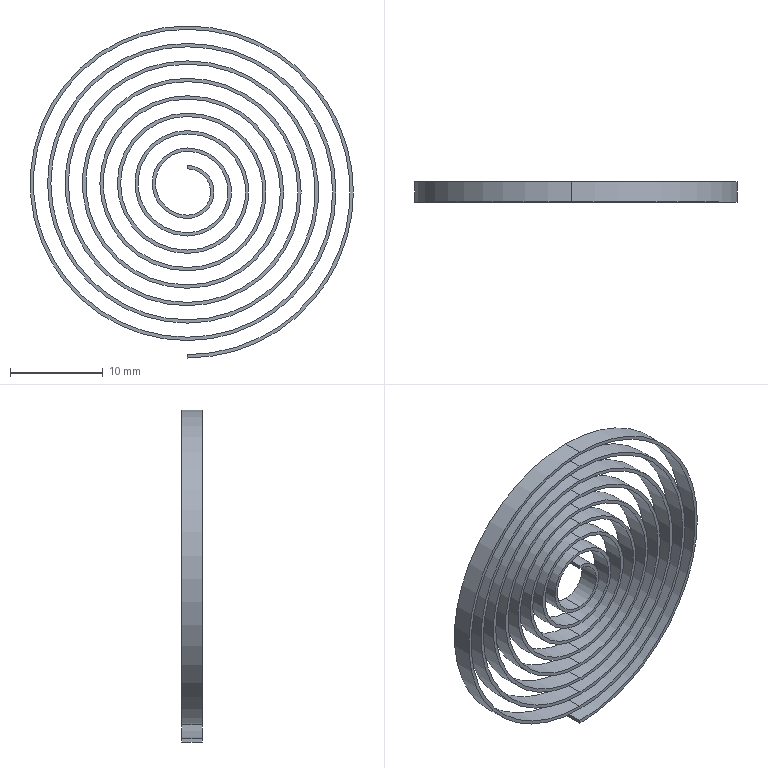Part | SolidWorks | features ExtruThin 1 | 1 solid | 38 faces | box 34.782 x 2.18 x 35.72 mm | volume 426.683 mm3 | cylinder 34 | plane 4 | commonest cylinder face diameters 5 x1 5.72 x1 6.875 x1 7.595 x1 8.75 x1 9.47 x1
STEP:
#1=CARTESIAN_POINT('',(0.,0.,17.86));
#2=VERTEX_POINT('',#1);
#3=CARTESIAN_POINT('',(0.,0.,-17.86));
#4=VERTEX_POINT('',#3);
#5=CARTESIAN_POINT('',(0.,0.,0.));
#6=DIRECTION('',(0.,1.,0.));
#7=DIRECTION('',(1.,0.,0.));
#8=AXIS2_PLACEMENT_3D('',#5,#6,#7);
#9=CIRCLE('',#8,17.86);
#10=EDGE_CURVE('',#2,#4,#9,.T.);
#11=ORIENTED_EDGE('',*,*,#10,.T.);
#12=CARTESIAN_POINT('',(0.,2.18,-17.86));
#13=VERTEX_POINT('',#12);
#14=CARTESIAN_POINT('',(0.,2.18,-17.86));
#15=DIRECTION('',(0.,-1.,0.));
#16=VECTOR('',#15,1000.);
#17=LINE('',#14,#16);
#18=EDGE_CURVE('',#13,#4,#17,.T.);
#19=ORIENTED_EDGE('',*,*,#18,.F.);
#20=CARTESIAN_POINT('',(0.,2.18,17.86));
#21=VERTEX_POINT('',#20);
#22=CARTESIAN_POINT('',(0.,2.18,0.));
#23=DIRECTION('',(0.,1.,0.));
#24=DIRECTION('',(1.,0.,0.));
#25=AXIS2_PLACEMENT_3D('',#22,#23,#24);
#26=CIRCLE('',#25,17.86);
#27=EDGE_CURVE('',#21,#13,#26,.T.);
#28=ORIENTED_EDGE('',*,*,#27,.F.);
#29=CARTESIAN_POINT('',(0.,2.18,17.86));
#30=DIRECTION('',(0.,-1.,0.));
#31=VECTOR('',#30,1000.);
#32=LINE('',#29,#31);
#33=EDGE_CURVE('',#21,#2,#32,.T.);
#34=ORIENTED_EDGE('',*,*,#33,.T.);
#35=EDGE_LOOP('',(#11,#19,#28,#34));
#36=FACE_OUTER_BOUND('',#35,.T.);
#37=CARTESIAN_POINT('',(0.,2.18,0.));
#38=DIRECTION('',(0.,-1.,0.));
#39=DIRECTION('',(0.,0.,-1.));
#40=AXIS2_PLACEMENT_3D('',#37,#38,#39);
#41=CYLINDRICAL_SURFACE('',#40,17.86);
#42=ADVANCED_FACE('',(#36),#41,.T.);
#43=CARTESIAN_POINT('',(0.,0.,-17.5));
#44=VERTEX_POINT('',#43);
#45=CARTESIAN_POINT('',(0.,0.,-17.5));
#46=DIRECTION('',(0.,0.,-1.));
#47=VECTOR('',#46,1000.);
#48=LINE('',#45,#47);
#49=EDGE_CURVE('',#44,#4,#48,.T.);
#50=ORIENTED_EDGE('',*,*,#49,.F.);
#51=CARTESIAN_POINT('',(0.,2.18,-17.5));
#52=VERTEX_POINT('',#51);
#53=CARTESIAN_POINT('',(0.,2.18,-17.5));
#54=DIRECTION('',(0.,-1.,0.));
#55=VECTOR('',#54,1000.);
#56=LINE('',#53,#55);
#57=EDGE_CURVE('',#52,#44,#56,.T.);
#58=ORIENTED_EDGE('',*,*,#57,.F.);
#59=CARTESIAN_POINT('',(0.,2.18,-17.5));
#60=DIRECTION('',(0.,0.,-1.));
#61=VECTOR('',#60,1000.);
#62=LINE('',#59,#61);
#63=EDGE_CURVE('',#52,#13,#62,.T.);
#64=ORIENTED_EDGE('',*,*,#63,.T.);
#65=ORIENTED_EDGE('',*,*,#18,.T.);
#66=EDGE_LOOP('',(#50,#58,#64,#65));
#67=FACE_OUTER_BOUND('',#66,.T.);
#68=CARTESIAN_POINT('',(0.,2.18,-17.5));
#69=DIRECTION('',(-1.,0.,0.));
#70=DIRECTION('',(0.,0.,1.));
#71=AXIS2_PLACEMENT_3D('',#68,#69,#70);
#72=PLANE('',#71);
#73=ADVANCED_FACE('',(#67),#72,.T.);
#74=CARTESIAN_POINT('',(0.,0.,17.5));
#75=VERTEX_POINT('',#74);
#76=CARTESIAN_POINT('',(0.,0.,0.));
#77=DIRECTION('',(0.,1.,0.));
#78=DIRECTION('',(0.,0.,1.));
#79=AXIS2_PLACEMENT_3D('',#76,#77,#78);
#80=CIRCLE('',#79,17.5);
#81=EDGE_CURVE('',#75,#44,#80,.T.);
#82=ORIENTED_EDGE('',*,*,#81,.F.);
#83=CARTESIAN_POINT('',(0.,2.18,17.5));
#84=VERTEX_POINT('',#83);
#85=CARTESIAN_POINT('',(0.,2.18,17.5));
#86=DIRECTION('',(0.,-1.,0.));
#87=VECTOR('',#86,1000.);
#88=LINE('',#85,#87);
#89=EDGE_CURVE('',#84,#75,#88,.T.);
#90=ORIENTED_EDGE('',*,*,#89,.F.);
#91=CARTESIAN_POINT('',(0.,2.18,0.));
#92=DIRECTION('',(0.,1.,0.));
#93=DIRECTION('',(0.,0.,1.));
#94=AXIS2_PLACEMENT_3D('',#91,#92,#93);
#95=CIRCLE('',#94,17.5);
#96=EDGE_CURVE('',#84,#52,#95,.T.);
#97=ORIENTED_EDGE('',*,*,#96,.T.);
#98=ORIENTED_EDGE('',*,*,#57,.T.);
#99=EDGE_LOOP('',(#82,#90,#97,#98));
#100=FACE_OUTER_BOUND('',#99,.T.);
#101=CARTESIAN_POINT('',(0.,2.18,0.));
#102=DIRECTION('',(0.,-1.,0.));
#103=DIRECTION('',(0.,0.,-1.));
#104=AXIS2_PLACEMENT_3D('',#101,#102,#103);
#105=CYLINDRICAL_SURFACE('',#104,17.5);
#106=ADVANCED_FACE('',(#100),#105,.F.);
#107=CARTESIAN_POINT('',(0.,0.,-15.625));
#108=VERTEX_POINT('',#107);
#109=CARTESIAN_POINT('',(0.,0.,0.9375));
#110=DIRECTION('',(0.,1.,0.));
#111=DIRECTION('',(0.,0.,1.));
#112=AXIS2_PLACEMENT_3D('',#109,#110,#111);
#113=CIRCLE('',#112,16.562);
#114=EDGE_CURVE('',#108,#75,#113,.T.);
#115=ORIENTED_EDGE('',*,*,#114,.F.);
#116=CARTESIAN_POINT('',(0.,2.18,-15.625));
#117=VERTEX_POINT('',#116);
#118=CARTESIAN_POINT('',(0.,2.18,-15.625));
#119=DIRECTION('',(0.,-1.,0.));
#120=VECTOR('',#119,1000.);
#121=LINE('',#118,#120);
#122=EDGE_CURVE('',#117,#108,#121,.T.);
#123=ORIENTED_EDGE('',*,*,#122,.F.);
#124=CARTESIAN_POINT('',(0.,2.18,0.9375));
#125=DIRECTION('',(0.,1.,0.));
#126=DIRECTION('',(0.,0.,1.));
#127=AXIS2_PLACEMENT_3D('',#124,#125,#126);
#128=CIRCLE('',#127,16.562);
#129=EDGE_CURVE('',#117,#84,#128,.T.);
#130=ORIENTED_EDGE('',*,*,#129,.T.);
#131=ORIENTED_EDGE('',*,*,#89,.T.);
#132=EDGE_LOOP('',(#115,#123,#130,#131));
#133=FACE_OUTER_BOUND('',#132,.T.);
#134=CARTESIAN_POINT('',(0.,2.18,0.9375));
#135=DIRECTION('',(0.,-1.,0.));
#136=DIRECTION('',(0.,0.,-1.));
#137=AXIS2_PLACEMENT_3D('',#134,#135,#136);
#138=CYLINDRICAL_SURFACE('',#137,16.562);
#139=ADVANCED_FACE('',(#133),#138,.F.);
#140=CARTESIAN_POINT('',(0.,0.,15.625));
#141=VERTEX_POINT('',#140);
#142=CARTESIAN_POINT('',(0.,0.,0.));
#143=DIRECTION('',(0.,1.,0.));
#144=DIRECTION('',(0.,0.,1.));
#145=AXIS2_PLACEMENT_3D('',#142,#143,#144);
#146=CIRCLE('',#145,15.625);
#147=EDGE_CURVE('',#141,#108,#146,.T.);
#148=ORIENTED_EDGE('',*,*,#147,.F.);
#149=CARTESIAN_POINT('',(0.,2.18,15.625));
#150=VERTEX_POINT('',#149);
#151=CARTESIAN_POINT('',(0.,2.18,15.625));
#152=DIRECTION('',(0.,-1.,0.));
#153=VECTOR('',#152,1000.);
#154=LINE('',#151,#153);
#155=EDGE_CURVE('',#150,#141,#154,.T.);
#156=ORIENTED_EDGE('',*,*,#155,.F.);
#157=CARTESIAN_POINT('',(0.,2.18,0.));
#158=DIRECTION('',(0.,1.,0.));
#159=DIRECTION('',(0.,0.,1.));
#160=AXIS2_PLACEMENT_3D('',#157,#158,#159);
#161=CIRCLE('',#160,15.625);
#162=EDGE_CURVE('',#150,#117,#161,.T.);
#163=ORIENTED_EDGE('',*,*,#162,.T.);
#164=ORIENTED_EDGE('',*,*,#122,.T.);
#165=EDGE_LOOP('',(#148,#156,#163,#164));
#166=FACE_OUTER_BOUND('',#165,.T.);
#167=CARTESIAN_POINT('',(0.,2.18,0.));
#168=DIRECTION('',(0.,-1.,0.));
#169=DIRECTION('',(0.,0.,-1.));
#170=AXIS2_PLACEMENT_3D('',#167,#168,#169);
#171=CYLINDRICAL_SURFACE('',#170,15.625);
#172=ADVANCED_FACE('',(#166),#171,.F.);
#173=CARTESIAN_POINT('',(0.,0.,-13.75));
#174=VERTEX_POINT('',#173);
#175=CARTESIAN_POINT('',(0.,0.,0.9375));
#176=DIRECTION('',(0.,1.,0.));
#177=DIRECTION('',(0.,0.,1.));
#178=AXIS2_PLACEMENT_3D('',#175,#176,#177);
#179=CIRCLE('',#178,14.687);
#180=EDGE_CURVE('',#174,#141,#179,.T.);
#181=ORIENTED_EDGE('',*,*,#180,.F.);
#182=CARTESIAN_POINT('',(0.,2.18,-13.75));
#183=VERTEX_POINT('',#182);
#184=CARTESIAN_POINT('',(0.,2.18,-13.75));
#185=DIRECTION('',(0.,-1.,0.));
#186=VECTOR('',#185,1000.);
#187=LINE('',#184,#186);
#188=EDGE_CURVE('',#183,#174,#187,.T.);
#189=ORIENTED_EDGE('',*,*,#188,.F.);
#190=CARTESIAN_POINT('',(0.,2.18,0.9375));
#191=DIRECTION('',(0.,1.,0.));
#192=DIRECTION('',(0.,0.,1.));
#193=AXIS2_PLACEMENT_3D('',#190,#191,#192);
#194=CIRCLE('',#193,14.687);
#195=EDGE_CURVE('',#183,#150,#194,.T.);
#196=ORIENTED_EDGE('',*,*,#195,.T.);
#197=ORIENTED_EDGE('',*,*,#155,.T.);
#198=EDGE_LOOP('',(#181,#189,#196,#197));
#199=FACE_OUTER_BOUND('',#198,.T.);
#200=CARTESIAN_POINT('',(0.,2.18,0.9375));
#201=DIRECTION('',(0.,-1.,0.));
#202=DIRECTION('',(0.,0.,-1.));
#203=AXIS2_PLACEMENT_3D('',#200,#201,#202);
#204=CYLINDRICAL_SURFACE('',#203,14.687);
#205=ADVANCED_FACE('',(#199),#204,.F.);
#206=CARTESIAN_POINT('',(0.,0.,13.75));
#207=VERTEX_POINT('',#206);
#208=CARTESIAN_POINT('',(0.,0.,0.));
#209=DIRECTION('',(0.,1.,0.));
#210=DIRECTION('',(0.,0.,1.));
#211=AXIS2_PLACEMENT_3D('',#208,#209,#210);
#212=CIRCLE('',#211,13.75);
#213=EDGE_CURVE('',#207,#174,#212,.T.);
#214=ORIENTED_EDGE('',*,*,#213,.F.);
#215=CARTESIAN_POINT('',(0.,2.18,13.75));
#216=VERTEX_POINT('',#215);
#217=CARTESIAN_POINT('',(0.,2.18,13.75));
#218=DIRECTION('',(0.,-1.,0.));
#219=VECTOR('',#218,1000.);
#220=LINE('',#217,#219);
#221=EDGE_CURVE('',#216,#207,#220,.T.);
#222=ORIENTED_EDGE('',*,*,#221,.F.);
#223=CARTESIAN_POINT('',(0.,2.18,0.));
#224=DIRECTION('',(0.,1.,0.));
#225=DIRECTION('',(0.,0.,1.));
#226=AXIS2_PLACEMENT_3D('',#223,#224,#225);
#227=CIRCLE('',#226,13.75);
#228=EDGE_CURVE('',#216,#183,#227,.T.);
#229=ORIENTED_EDGE('',*,*,#228,.T.);
#230=ORIENTED_EDGE('',*,*,#188,.T.);
#231=EDGE_LOOP('',(#214,#222,#229,#230));
#232=FACE_OUTER_BOUND('',#231,.T.);
#233=CARTESIAN_POINT('',(0.,2.18,0.));
#234=DIRECTION('',(0.,-1.,0.));
#235=DIRECTION('',(0.,0.,-1.));
#236=AXIS2_PLACEMENT_3D('',#233,#234,#235);
#237=CYLINDRICAL_SURFACE('',#236,13.75);
#238=ADVANCED_FACE('',(#232),#237,.F.);
#239=CARTESIAN_POINT('',(0.,0.,-11.875));
#240=VERTEX_POINT('',#239);
#241=CARTESIAN_POINT('',(0.,0.,0.9375));
#242=DIRECTION('',(0.,1.,0.));
#243=DIRECTION('',(0.,0.,1.));
#244=AXIS2_PLACEMENT_3D('',#241,#242,#243);
#245=CIRCLE('',#244,12.812);
#246=EDGE_CURVE('',#240,#207,#245,.T.);
#247=ORIENTED_EDGE('',*,*,#246,.F.);
#248=CARTESIAN_POINT('',(0.,2.18,-11.875));
#249=VERTEX_POINT('',#248);
#250=CARTESIAN_POINT('',(0.,2.18,-11.875));
#251=DIRECTION('',(0.,-1.,0.));
#252=VECTOR('',#251,1000.);
#253=LINE('',#250,#252);
#254=EDGE_CURVE('',#249,#240,#253,.T.);
#255=ORIENTED_EDGE('',*,*,#254,.F.);
#256=CARTESIAN_POINT('',(0.,2.18,0.9375));
#257=DIRECTION('',(0.,1.,0.));
#258=DIRECTION('',(0.,0.,1.));
#259=AXIS2_PLACEMENT_3D('',#256,#257,#258);
#260=CIRCLE('',#259,12.812);
#261=EDGE_CURVE('',#249,#216,#260,.T.);
#262=ORIENTED_EDGE('',*,*,#261,.T.);
#263=ORIENTED_EDGE('',*,*,#221,.T.);
#264=EDGE_LOOP('',(#247,#255,#262,#263));
#265=FACE_OUTER_BOUND('',#264,.T.);
#266=CARTESIAN_POINT('',(0.,2.18,0.9375));
#267=DIRECTION('',(0.,-1.,0.));
#268=DIRECTION('',(0.,0.,-1.));
#269=AXIS2_PLACEMENT_3D('',#266,#267,#268);
#270=CYLINDRICAL_SURFACE('',#269,12.812);
#271=ADVANCED_FACE('',(#265),#270,.F.);
#272=CARTESIAN_POINT('',(0.,0.,11.875));
#273=VERTEX_POINT('',#272);
#274=CARTESIAN_POINT('',(0.,0.,0.));
#275=DIRECTION('',(0.,1.,0.));
#276=DIRECTION('',(0.,0.,1.));
#277=AXIS2_PLACEMENT_3D('',#274,#275,#276);
#278=CIRCLE('',#277,11.875);
#279=EDGE_CURVE('',#273,#240,#278,.T.);
#280=ORIENTED_EDGE('',*,*,#279,.F.);
#281=CARTESIAN_POINT('',(0.,2.18,11.875));
#282=VERTEX_POINT('',#281);
#283=CARTESIAN_POINT('',(0.,2.18,11.875));
#284=DIRECTION('',(0.,-1.,0.));
#285=VECTOR('',#284,1000.);
#286=LINE('',#283,#285);
#287=EDGE_CURVE('',#282,#273,#286,.T.);
#288=ORIENTED_EDGE('',*,*,#287,.F.);
#289=CARTESIAN_POINT('',(0.,2.18,0.));
#290=DIRECTION('',(0.,1.,0.));
#291=DIRECTION('',(0.,0.,1.));
#292=AXIS2_PLACEMENT_3D('',#289,#290,#291);
#293=CIRCLE('',#292,11.875);
#294=EDGE_CURVE('',#282,#249,#293,.T.);
#295=ORIENTED_EDGE('',*,*,#294,.T.);
#296=ORIENTED_EDGE('',*,*,#254,.T.);
#297=EDGE_LOOP('',(#280,#288,#295,#296));
#298=FACE_OUTER_BOUND('',#297,.T.);
#299=CARTESIAN_POINT('',(0.,2.18,0.));
#300=DIRECTION('',(0.,-1.,0.));
#301=DIRECTION('',(0.,0.,-1.));
#302=AXIS2_PLACEMENT_3D('',#299,#300,#301);
#303=CYLINDRICAL_SURFACE('',#302,11.875);
#304=ADVANCED_FACE('',(#298),#303,.F.);
#305=CARTESIAN_POINT('',(0.,0.,-10.));
#306=VERTEX_POINT('',#305);
#307=CARTESIAN_POINT('',(0.,0.,0.9375));
#308=DIRECTION('',(0.,1.,0.));
#309=DIRECTION('',(0.,0.,1.));
#310=AXIS2_PLACEMENT_3D('',#307,#308,#309);
#311=CIRCLE('',#310,10.938);
#312=EDGE_CURVE('',#306,#273,#311,.T.);
#313=ORIENTED_EDGE('',*,*,#312,.F.);
#314=CARTESIAN_POINT('',(0.,2.18,-10.));
#315=VERTEX_POINT('',#314);
#316=CARTESIAN_POINT('',(0.,2.18,-10.));
#317=DIRECTION('',(0.,-1.,0.));
#318=VECTOR('',#317,1000.);
#319=LINE('',#316,#318);
#320=EDGE_CURVE('',#315,#306,#319,.T.);
#321=ORIENTED_EDGE('',*,*,#320,.F.);
#322=CARTESIAN_POINT('',(0.,2.18,0.9375));
#323=DIRECTION('',(0.,1.,0.));
#324=DIRECTION('',(0.,0.,1.));
#325=AXIS2_PLACEMENT_3D('',#322,#323,#324);
#326=CIRCLE('',#325,10.938);
#327=EDGE_CURVE('',#315,#282,#326,.T.);
#328=ORIENTED_EDGE('',*,*,#327,.T.);
#329=ORIENTED_EDGE('',*,*,#287,.T.);
#330=EDGE_LOOP('',(#313,#321,#328,#329));
#331=FACE_OUTER_BOUND('',#330,.T.);
#332=CARTESIAN_POINT('',(0.,2.18,0.9375));
#333=DIRECTION('',(0.,-1.,0.));
#334=DIRECTION('',(0.,0.,-1.));
#335=AXIS2_PLACEMENT_3D('',#332,#333,#334);
#336=CYLINDRICAL_SURFACE('',#335,10.938);
#337=ADVANCED_FACE('',(#331),#336,.F.);
#338=CARTESIAN_POINT('',(0.,0.,10.));
#339=VERTEX_POINT('',#338);
#340=CARTESIAN_POINT('',(0.,0.,0.));
#341=DIRECTION('',(0.,1.,0.));
#342=DIRECTION('',(0.,0.,1.));
#343=AXIS2_PLACEMENT_3D('',#340,#341,#342);
#344=CIRCLE('',#343,10.);
#345=EDGE_CURVE('',#339,#306,#344,.T.);
#346=ORIENTED_EDGE('',*,*,#345,.F.);
#347=CARTESIAN_POINT('',(0.,2.18,10.));
#348=VERTEX_POINT('',#347);
#349=CARTESIAN_POINT('',(0.,2.18,10.));
#350=DIRECTION('',(0.,-1.,0.));
#351=VECTOR('',#350,1000.);
#352=LINE('',#349,#351);
#353=EDGE_CURVE('',#348,#339,#352,.T.);
#354=ORIENTED_EDGE('',*,*,#353,.F.);
#355=CARTESIAN_POINT('',(0.,2.18,0.));
#356=DIRECTION('',(0.,1.,0.));
#357=DIRECTION('',(0.,0.,1.));
#358=AXIS2_PLACEMENT_3D('',#355,#356,#357);
#359=CIRCLE('',#358,10.);
#360=EDGE_CURVE('',#348,#315,#359,.T.);
#361=ORIENTED_EDGE('',*,*,#360,.T.);
#362=ORIENTED_EDGE('',*,*,#320,.T.);
#363=EDGE_LOOP('',(#346,#354,#361,#362));
#364=FACE_OUTER_BOUND('',#363,.T.);
#365=CARTESIAN_POINT('',(0.,2.18,0.));
#366=DIRECTION('',(0.,-1.,0.));
#367=DIRECTION('',(0.,0.,-1.));
#368=AXIS2_PLACEMENT_3D('',#365,#366,#367);
#369=CYLINDRICAL_SURFACE('',#368,10.);
#370=ADVANCED_FACE('',(#364),#369,.F.);
#371=CARTESIAN_POINT('',(0.,0.,-8.125));
#372=VERTEX_POINT('',#371);
#373=CARTESIAN_POINT('',(0.,0.,0.9375));
#374=DIRECTION('',(0.,1.,0.));
#375=DIRECTION('',(0.,0.,1.));
#376=AXIS2_PLACEMENT_3D('',#373,#374,#375);
#377=CIRCLE('',#376,9.062);
#378=EDGE_CURVE('',#372,#339,#377,.T.);
#379=ORIENTED_EDGE('',*,*,#378,.F.);
#380=CARTESIAN_POINT('',(0.,2.18,-8.125));
#381=VERTEX_POINT('',#380);
#382=CARTESIAN_POINT('',(0.,2.18,-8.125));
#383=DIRECTION('',(0.,-1.,0.));
#384=VECTOR('',#383,1000.);
#385=LINE('',#382,#384);
#386=EDGE_CURVE('',#381,#372,#385,.T.);
#387=ORIENTED_EDGE('',*,*,#386,.F.);
#388=CARTESIAN_POINT('',(0.,2.18,0.9375));
#389=DIRECTION('',(0.,1.,0.));
#390=DIRECTION('',(0.,0.,1.));
#391=AXIS2_PLACEMENT_3D('',#388,#389,#390);
#392=CIRCLE('',#391,9.062);
#393=EDGE_CURVE('',#381,#348,#392,.T.);
#394=ORIENTED_EDGE('',*,*,#393,.T.);
#395=ORIENTED_EDGE('',*,*,#353,.T.);
#396=EDGE_LOOP('',(#379,#387,#394,#395));
#397=FACE_OUTER_BOUND('',#396,.T.);
#398=CARTESIAN_POINT('',(0.,2.18,0.9375));
#399=DIRECTION('',(0.,-1.,0.));
#400=DIRECTION('',(0.,0.,-1.));
#401=AXIS2_PLACEMENT_3D('',#398,#399,#400);
#402=CYLINDRICAL_SURFACE('',#401,9.062);
#403=ADVANCED_FACE('',(#397),#402,.F.);
#404=CARTESIAN_POINT('',(0.,0.,8.125));
#405=VERTEX_POINT('',#404);
#406=CARTESIAN_POINT('',(0.,0.,0.));
#407=DIRECTION('',(0.,1.,0.));
#408=DIRECTION('',(0.,0.,1.));
#409=AXIS2_PLACEMENT_3D('',#406,#407,#408);
#410=CIRCLE('',#409,8.125);
#411=EDGE_CURVE('',#405,#372,#410,.T.);
#412=ORIENTED_EDGE('',*,*,#411,.F.);
#413=CARTESIAN_POINT('',(0.,2.18,8.125));
#414=VERTEX_POINT('',#413);
#415=CARTESIAN_POINT('',(0.,2.18,8.125));
#416=DIRECTION('',(0.,-1.,0.));
#417=VECTOR('',#416,1000.);
#418=LINE('',#415,#417);
#419=EDGE_CURVE('',#414,#405,#418,.T.);
#420=ORIENTED_EDGE('',*,*,#419,.F.);
#421=CARTESIAN_POINT('',(0.,2.18,0.));
#422=DIRECTION('',(0.,1.,0.));
#423=DIRECTION('',(0.,0.,1.));
#424=AXIS2_PLACEMENT_3D('',#421,#422,#423);
#425=CIRCLE('',#424,8.125);
#426=EDGE_CURVE('',#414,#381,#425,.T.);
#427=ORIENTED_EDGE('',*,*,#426,.T.);
#428=ORIENTED_EDGE('',*,*,#386,.T.);
#429=EDGE_LOOP('',(#412,#420,#427,#428));
#430=FACE_OUTER_BOUND('',#429,.T.);
#431=CARTESIAN_POINT('',(0.,2.18,0.));
#432=DIRECTION('',(0.,-1.,0.));
#433=DIRECTION('',(0.,0.,-1.));
#434=AXIS2_PLACEMENT_3D('',#431,#432,#433);
#435=CYLINDRICAL_SURFACE('',#434,8.125);
#436=ADVANCED_FACE('',(#430),#435,.F.);
#437=CARTESIAN_POINT('',(0.,0.,-6.25));
#438=VERTEX_POINT('',#437);
#439=CARTESIAN_POINT('',(0.,0.,0.9375));
#440=DIRECTION('',(0.,1.,0.));
#441=DIRECTION('',(0.,0.,1.));
#442=AXIS2_PLACEMENT_3D('',#439,#440,#441);
#443=CIRCLE('',#442,7.188);
#444=EDGE_CURVE('',#438,#405,#443,.T.);
#445=ORIENTED_EDGE('',*,*,#444,.F.);
#446=CARTESIAN_POINT('',(0.,2.18,-6.25));
#447=VERTEX_POINT('',#446);
#448=CARTESIAN_POINT('',(0.,2.18,-6.25));
#449=DIRECTION('',(0.,-1.,0.));
#450=VECTOR('',#449,1000.);
#451=LINE('',#448,#450);
#452=EDGE_CURVE('',#447,#438,#451,.T.);
#453=ORIENTED_EDGE('',*,*,#452,.F.);
#454=CARTESIAN_POINT('',(0.,2.18,0.9375));
#455=DIRECTION('',(0.,1.,0.));
#456=DIRECTION('',(0.,0.,1.));
#457=AXIS2_PLACEMENT_3D('',#454,#455,#456);
#458=CIRCLE('',#457,7.188);
#459=EDGE_CURVE('',#447,#414,#458,.T.);
#460=ORIENTED_EDGE('',*,*,#459,.T.);
#461=ORIENTED_EDGE('',*,*,#419,.T.);
#462=EDGE_LOOP('',(#445,#453,#460,#461));
#463=FACE_OUTER_BOUND('',#462,.T.);
#464=CARTESIAN_POINT('',(0.,2.18,0.9375));
#465=DIRECTION('',(0.,-1.,0.));
#466=DIRECTION('',(0.,0.,-1.));
#467=AXIS2_PLACEMENT_3D('',#464,#465,#466);
#468=CYLINDRICAL_SURFACE('',#467,7.188);
#469=ADVANCED_FACE('',(#463),#468,.F.);
#470=CARTESIAN_POINT('',(0.,0.,6.25));
#471=VERTEX_POINT('',#470);
#472=CARTESIAN_POINT('',(0.,0.,0.));
#473=DIRECTION('',(0.,1.,0.));
#474=DIRECTION('',(0.,0.,1.));
#475=AXIS2_PLACEMENT_3D('',#472,#473,#474);
#476=CIRCLE('',#475,6.25);
#477=EDGE_CURVE('',#471,#438,#476,.T.);
#478=ORIENTED_EDGE('',*,*,#477,.F.);
#479=CARTESIAN_POINT('',(0.,2.18,6.25));
#480=VERTEX_POINT('',#479);
#481=CARTESIAN_POINT('',(0.,2.18,6.25));
#482=DIRECTION('',(0.,-1.,0.));
#483=VECTOR('',#482,1000.);
#484=LINE('',#481,#483);
#485=EDGE_CURVE('',#480,#471,#484,.T.);
#486=ORIENTED_EDGE('',*,*,#485,.F.);
#487=CARTESIAN_POINT('',(0.,2.18,0.));
#488=DIRECTION('',(0.,1.,0.));
#489=DIRECTION('',(0.,0.,1.));
#490=AXIS2_PLACEMENT_3D('',#487,#488,#489);
#491=CIRCLE('',#490,6.25);
#492=EDGE_CURVE('',#480,#447,#491,.T.);
#493=ORIENTED_EDGE('',*,*,#492,.T.);
#494=ORIENTED_EDGE('',*,*,#452,.T.);
#495=EDGE_LOOP('',(#478,#486,#493,#494));
#496=FACE_OUTER_BOUND('',#495,.T.);
#497=CARTESIAN_POINT('',(0.,2.18,0.));
#498=DIRECTION('',(0.,-1.,0.));
#499=DIRECTION('',(0.,0.,-1.));
#500=AXIS2_PLACEMENT_3D('',#497,#498,#499);
#501=CYLINDRICAL_SURFACE('',#500,6.25);
#502=ADVANCED_FACE('',(#496),#501,.F.);
#503=CARTESIAN_POINT('',(0.,0.,-4.375));
#504=VERTEX_POINT('',#503);
#505=CARTESIAN_POINT('',(0.,0.,0.9375));
#506=DIRECTION('',(0.,1.,0.));
#507=DIRECTION('',(0.,0.,1.));
#508=AXIS2_PLACEMENT_3D('',#505,#506,#507);
#509=CIRCLE('',#508,5.312);
#510=EDGE_CURVE('',#504,#471,#509,.T.);
#511=ORIENTED_EDGE('',*,*,#510,.F.);
#512=CARTESIAN_POINT('',(0.,2.18,-4.375));
#513=VERTEX_POINT('',#512);
#514=CARTESIAN_POINT('',(0.,2.18,-4.375));
#515=DIRECTION('',(0.,-1.,0.));
#516=VECTOR('',#515,1000.);
#517=LINE('',#514,#516);
#518=EDGE_CURVE('',#513,#504,#517,.T.);
#519=ORIENTED_EDGE('',*,*,#518,.F.);
#520=CARTESIAN_POINT('',(0.,2.18,0.9375));
#521=DIRECTION('',(0.,1.,0.));
#522=DIRECTION('',(0.,0.,1.));
#523=AXIS2_PLACEMENT_3D('',#520,#521,#522);
#524=CIRCLE('',#523,5.312);
#525=EDGE_CURVE('',#513,#480,#524,.T.);
#526=ORIENTED_EDGE('',*,*,#525,.T.);
#527=ORIENTED_EDGE('',*,*,#485,.T.);
#528=EDGE_LOOP('',(#511,#519,#526,#527));
#529=FACE_OUTER_BOUND('',#528,.T.);
#530=CARTESIAN_POINT('',(0.,2.18,0.9375));
#531=DIRECTION('',(0.,-1.,0.));
#532=DIRECTION('',(0.,0.,-1.));
#533=AXIS2_PLACEMENT_3D('',#530,#531,#532);
#534=CYLINDRICAL_SURFACE('',#533,5.312);
#535=ADVANCED_FACE('',(#529),#534,.F.);
#536=CARTESIAN_POINT('',(0.,0.,4.375));
#537=VERTEX_POINT('',#536);
#538=CARTESIAN_POINT('',(0.,0.,0.));
#539=DIRECTION('',(0.,1.,0.));
#540=DIRECTION('',(0.,0.,1.));
#541=AXIS2_PLACEMENT_3D('',#538,#539,#540);
#542=CIRCLE('',#541,4.375);
#543=EDGE_CURVE('',#537,#504,#542,.T.);
#544=ORIENTED_EDGE('',*,*,#543,.F.);
#545=CARTESIAN_POINT('',(0.,2.18,4.375));
#546=VERTEX_POINT('',#545);
#547=CARTESIAN_POINT('',(0.,2.18,4.375));
#548=DIRECTION('',(0.,-1.,0.));
#549=VECTOR('',#548,1000.);
#550=LINE('',#547,#549);
#551=EDGE_CURVE('',#546,#537,#550,.T.);
#552=ORIENTED_EDGE('',*,*,#551,.F.);
#553=CARTESIAN_POINT('',(0.,2.18,0.));
#554=DIRECTION('',(0.,1.,0.));
#555=DIRECTION('',(0.,0.,1.));
#556=AXIS2_PLACEMENT_3D('',#553,#554,#555);
#557=CIRCLE('',#556,4.375);
#558=EDGE_CURVE('',#546,#513,#557,.T.);
#559=ORIENTED_EDGE('',*,*,#558,.T.);
#560=ORIENTED_EDGE('',*,*,#518,.T.);
#561=EDGE_LOOP('',(#544,#552,#559,#560));
#562=FACE_OUTER_BOUND('',#561,.T.);
#563=CARTESIAN_POINT('',(0.,2.18,0.));
#564=DIRECTION('',(0.,-1.,0.));
#565=DIRECTION('',(0.,0.,-1.));
#566=AXIS2_PLACEMENT_3D('',#563,#564,#565);
#567=CYLINDRICAL_SURFACE('',#566,4.375);
#568=ADVANCED_FACE('',(#562),#567,.F.);
#569=CARTESIAN_POINT('',(0.,0.,-2.5));
#570=VERTEX_POINT('',#569);
#571=CARTESIAN_POINT('',(0.,0.,0.9375));
#572=DIRECTION('',(0.,1.,0.));
#573=DIRECTION('',(0.,0.,1.));
#574=AXIS2_PLACEMENT_3D('',#571,#572,#573);
#575=CIRCLE('',#574,3.438);
#576=EDGE_CURVE('',#570,#537,#575,.T.);
#577=ORIENTED_EDGE('',*,*,#576,.F.);
#578=CARTESIAN_POINT('',(0.,2.18,-2.5));
#579=VERTEX_POINT('',#578);
#580=CARTESIAN_POINT('',(0.,2.18,-2.5));
#581=DIRECTION('',(0.,-1.,0.));
#582=VECTOR('',#581,1000.);
#583=LINE('',#580,#582);
#584=EDGE_CURVE('',#579,#570,#583,.T.);
#585=ORIENTED_EDGE('',*,*,#584,.F.);
#586=CARTESIAN_POINT('',(0.,2.18,0.9375));
#587=DIRECTION('',(0.,1.,0.));
#588=DIRECTION('',(0.,0.,1.));
#589=AXIS2_PLACEMENT_3D('',#586,#587,#588);
#590=CIRCLE('',#589,3.438);
#591=EDGE_CURVE('',#579,#546,#590,.T.);
#592=ORIENTED_EDGE('',*,*,#591,.T.);
#593=ORIENTED_EDGE('',*,*,#551,.T.);
#594=EDGE_LOOP('',(#577,#585,#592,#593));
#595=FACE_OUTER_BOUND('',#594,.T.);
#596=CARTESIAN_POINT('',(0.,2.18,0.9375));
#597=DIRECTION('',(0.,-1.,0.));
#598=DIRECTION('',(0.,0.,-1.));
#599=AXIS2_PLACEMENT_3D('',#596,#597,#598);
#600=CYLINDRICAL_SURFACE('',#599,3.438);
#601=ADVANCED_FACE('',(#595),#600,.F.);
#602=CARTESIAN_POINT('',(0.,0.,2.5));
#603=VERTEX_POINT('',#602);
#604=CARTESIAN_POINT('',(0.,0.,0.));
#605=DIRECTION('',(0.,1.,0.));
#606=DIRECTION('',(0.,0.,1.));
#607=AXIS2_PLACEMENT_3D('',#604,#605,#606);
#608=CIRCLE('',#607,2.5);
#609=EDGE_CURVE('',#603,#570,#608,.T.);
#610=ORIENTED_EDGE('',*,*,#609,.F.);
#611=CARTESIAN_POINT('',(0.,2.18,2.5));
#612=VERTEX_POINT('',#611);
#613=CARTESIAN_POINT('',(0.,2.18,2.5));
#614=DIRECTION('',(0.,-1.,0.));
#615=VECTOR('',#614,1000.);
#616=LINE('',#613,#615);
#617=EDGE_CURVE('',#612,#603,#616,.T.);
#618=ORIENTED_EDGE('',*,*,#617,.F.);
#619=CARTESIAN_POINT('',(0.,2.18,0.));
#620=DIRECTION('',(0.,1.,0.));
#621=DIRECTION('',(0.,0.,1.));
#622=AXIS2_PLACEMENT_3D('',#619,#620,#621);
#623=CIRCLE('',#622,2.5);
#624=EDGE_CURVE('',#612,#579,#623,.T.);
#625=ORIENTED_EDGE('',*,*,#624,.T.);
#626=ORIENTED_EDGE('',*,*,#584,.T.);
#627=EDGE_LOOP('',(#610,#618,#625,#626));
#628=FACE_OUTER_BOUND('',#627,.T.);
#629=CARTESIAN_POINT('',(0.,2.18,0.));
#630=DIRECTION('',(0.,-1.,0.));
#631=DIRECTION('',(0.,0.,-1.));
#632=AXIS2_PLACEMENT_3D('',#629,#630,#631);
#633=CYLINDRICAL_SURFACE('',#632,2.5);
#634=ADVANCED_FACE('',(#628),#633,.F.);
#635=CARTESIAN_POINT('',(0.,0.,2.86));
#636=VERTEX_POINT('',#635);
#637=CARTESIAN_POINT('',(0.,0.,2.86));
#638=DIRECTION('',(0.,0.,-1.));
#639=VECTOR('',#638,1000.);
#640=LINE('',#637,#639);
#641=EDGE_CURVE('',#636,#603,#640,.T.);
#642=ORIENTED_EDGE('',*,*,#641,.F.);
#643=CARTESIAN_POINT('',(0.,2.18,2.86));
#644=VERTEX_POINT('',#643);
#645=CARTESIAN_POINT('',(0.,2.18,2.86));
#646=DIRECTION('',(0.,-1.,0.));
#647=VECTOR('',#646,1000.);
#648=LINE('',#645,#647);
#649=EDGE_CURVE('',#644,#636,#648,.T.);
#650=ORIENTED_EDGE('',*,*,#649,.F.);
#651=CARTESIAN_POINT('',(0.,2.18,2.86));
#652=DIRECTION('',(0.,0.,-1.));
#653=VECTOR('',#652,1000.);
#654=LINE('',#651,#653);
#655=EDGE_CURVE('',#644,#612,#654,.T.);
#656=ORIENTED_EDGE('',*,*,#655,.T.);
#657=ORIENTED_EDGE('',*,*,#617,.T.);
#658=EDGE_LOOP('',(#642,#650,#656,#657));
#659=FACE_OUTER_BOUND('',#658,.T.);
#660=CARTESIAN_POINT('',(0.,2.18,2.86));
#661=DIRECTION('',(-1.,0.,0.));
#662=DIRECTION('',(0.,0.,1.));
#663=AXIS2_PLACEMENT_3D('',#660,#661,#662);
#664=PLANE('',#663);
#665=ADVANCED_FACE('',(#659),#664,.T.);
#666=CARTESIAN_POINT('',(0.,0.,-2.86));
#667=VERTEX_POINT('',#666);
#668=CARTESIAN_POINT('',(0.,0.,0.));
#669=DIRECTION('',(0.,1.,0.));
#670=DIRECTION('',(1.,0.,0.));
#671=AXIS2_PLACEMENT_3D('',#668,#669,#670);
#672=CIRCLE('',#671,2.86);
#673=EDGE_CURVE('',#636,#667,#672,.T.);
#674=ORIENTED_EDGE('',*,*,#673,.T.);
#675=CARTESIAN_POINT('',(0.,2.18,-2.86));
#676=VERTEX_POINT('',#675);
#677=CARTESIAN_POINT('',(0.,2.18,-2.86));
#678=DIRECTION('',(0.,-1.,0.));
#679=VECTOR('',#678,1000.);
#680=LINE('',#677,#679);
#681=EDGE_CURVE('',#676,#667,#680,.T.);
#682=ORIENTED_EDGE('',*,*,#681,.F.);
#683=CARTESIAN_POINT('',(0.,2.18,0.));
#684=DIRECTION('',(0.,1.,0.));
#685=DIRECTION('',(1.,0.,0.));
#686=AXIS2_PLACEMENT_3D('',#683,#684,#685);
#687=CIRCLE('',#686,2.86);
#688=EDGE_CURVE('',#644,#676,#687,.T.);
#689=ORIENTED_EDGE('',*,*,#688,.F.);
#690=ORIENTED_EDGE('',*,*,#649,.T.);
#691=EDGE_LOOP('',(#674,#682,#689,#690));
#692=FACE_OUTER_BOUND('',#691,.T.);
#693=CARTESIAN_POINT('',(0.,2.18,0.));
#694=DIRECTION('',(0.,-1.,0.));
#695=DIRECTION('',(0.,0.,-1.));
#696=AXIS2_PLACEMENT_3D('',#693,#694,#695);
#697=CYLINDRICAL_SURFACE('',#696,2.86);
#698=ADVANCED_FACE('',(#692),#697,.T.);
#699=CARTESIAN_POINT('',(0.,0.,4.735));
#700=VERTEX_POINT('',#699);
#701=CARTESIAN_POINT('',(0.,0.,0.9375));
#702=DIRECTION('',(0.,1.,0.));
#703=DIRECTION('',(1.,0.,0.));
#704=AXIS2_PLACEMENT_3D('',#701,#702,#703);
#705=CIRCLE('',#704,3.798);
#706=EDGE_CURVE('',#667,#700,#705,.T.);
#707=ORIENTED_EDGE('',*,*,#706,.T.);
#708=CARTESIAN_POINT('',(0.,2.18,4.735));
#709=VERTEX_POINT('',#708);
#710=CARTESIAN_POINT('',(0.,2.18,4.735));
#711=DIRECTION('',(0.,-1.,0.));
#712=VECTOR('',#711,1000.);
#713=LINE('',#710,#712);
#714=EDGE_CURVE('',#709,#700,#713,.T.);
#715=ORIENTED_EDGE('',*,*,#714,.F.);
#716=CARTESIAN_POINT('',(0.,2.18,0.9375));
#717=DIRECTION('',(0.,1.,0.));
#718=DIRECTION('',(1.,0.,0.));
#719=AXIS2_PLACEMENT_3D('',#716,#717,#718);
#720=CIRCLE('',#719,3.798);
#721=EDGE_CURVE('',#676,#709,#720,.T.);
#722=ORIENTED_EDGE('',*,*,#721,.F.);
#723=ORIENTED_EDGE('',*,*,#681,.T.);
#724=EDGE_LOOP('',(#707,#715,#722,#723));
#725=FACE_OUTER_BOUND('',#724,.T.);
#726=CARTESIAN_POINT('',(0.,2.18,0.9375));
#727=DIRECTION('',(0.,-1.,0.));
#728=DIRECTION('',(0.,0.,-1.));
#729=AXIS2_PLACEMENT_3D('',#726,#727,#728);
#730=CYLINDRICAL_SURFACE('',#729,3.798);
#731=ADVANCED_FACE('',(#725),#730,.T.);
#732=CARTESIAN_POINT('',(0.,0.,-4.735));
#733=VERTEX_POINT('',#732);
#734=CARTESIAN_POINT('',(0.,0.,0.));
#735=DIRECTION('',(0.,1.,0.));
#736=DIRECTION('',(1.,0.,0.));
#737=AXIS2_PLACEMENT_3D('',#734,#735,#736);
#738=CIRCLE('',#737,4.735);
#739=EDGE_CURVE('',#700,#733,#738,.T.);
#740=ORIENTED_EDGE('',*,*,#739,.T.);
#741=CARTESIAN_POINT('',(0.,2.18,-4.735));
#742=VERTEX_POINT('',#741);
#743=CARTESIAN_POINT('',(0.,2.18,-4.735));
#744=DIRECTION('',(0.,-1.,0.));
#745=VECTOR('',#744,1000.);
#746=LINE('',#743,#745);
#747=EDGE_CURVE('',#742,#733,#746,.T.);
#748=ORIENTED_EDGE('',*,*,#747,.F.);
#749=CARTESIAN_POINT('',(0.,2.18,0.));
#750=DIRECTION('',(0.,1.,0.));
#751=DIRECTION('',(1.,0.,0.));
#752=AXIS2_PLACEMENT_3D('',#749,#750,#751);
#753=CIRCLE('',#752,4.735);
#754=EDGE_CURVE('',#709,#742,#753,.T.);
#755=ORIENTED_EDGE('',*,*,#754,.F.);
#756=ORIENTED_EDGE('',*,*,#714,.T.);
#757=EDGE_LOOP('',(#740,#748,#755,#756));
#758=FACE_OUTER_BOUND('',#757,.T.);
#759=CARTESIAN_POINT('',(0.,2.18,0.));
#760=DIRECTION('',(0.,-1.,0.));
#761=DIRECTION('',(0.,0.,-1.));
#762=AXIS2_PLACEMENT_3D('',#759,#760,#761);
#763=CYLINDRICAL_SURFACE('',#762,4.735);
#764=ADVANCED_FACE('',(#758),#763,.T.);
#765=CARTESIAN_POINT('',(0.,0.,6.61));
#766=VERTEX_POINT('',#765);
#767=CARTESIAN_POINT('',(0.,0.,0.9375));
#768=DIRECTION('',(0.,1.,0.));
#769=DIRECTION('',(1.,0.,0.));
#770=AXIS2_PLACEMENT_3D('',#767,#768,#769);
#771=CIRCLE('',#770,5.673);
#772=EDGE_CURVE('',#733,#766,#771,.T.);
#773=ORIENTED_EDGE('',*,*,#772,.T.);
#774=CARTESIAN_POINT('',(0.,2.18,6.61));
#775=VERTEX_POINT('',#774);
#776=CARTESIAN_POINT('',(0.,2.18,6.61));
#777=DIRECTION('',(0.,-1.,0.));
#778=VECTOR('',#777,1000.);
#779=LINE('',#776,#778);
#780=EDGE_CURVE('',#775,#766,#779,.T.);
#781=ORIENTED_EDGE('',*,*,#780,.F.);
#782=CARTESIAN_POINT('',(0.,2.18,0.9375));
#783=DIRECTION('',(0.,1.,0.));
#784=DIRECTION('',(1.,0.,0.));
#785=AXIS2_PLACEMENT_3D('',#782,#783,#784);
#786=CIRCLE('',#785,5.673);
#787=EDGE_CURVE('',#742,#775,#786,.T.);
#788=ORIENTED_EDGE('',*,*,#787,.F.);
#789=ORIENTED_EDGE('',*,*,#747,.T.);
#790=EDGE_LOOP('',(#773,#781,#788,#789));
#791=FACE_OUTER_BOUND('',#790,.T.);
#792=CARTESIAN_POINT('',(0.,2.18,0.9375));
#793=DIRECTION('',(0.,-1.,0.));
#794=DIRECTION('',(0.,0.,-1.));
#795=AXIS2_PLACEMENT_3D('',#792,#793,#794);
#796=CYLINDRICAL_SURFACE('',#795,5.673);
#797=ADVANCED_FACE('',(#791),#796,.T.);
#798=CARTESIAN_POINT('',(0.,0.,-6.61));
#799=VERTEX_POINT('',#798);
#800=CARTESIAN_POINT('',(0.,0.,0.));
#801=DIRECTION('',(0.,1.,0.));
#802=DIRECTION('',(1.,0.,0.));
#803=AXIS2_PLACEMENT_3D('',#800,#801,#802);
#804=CIRCLE('',#803,6.61);
#805=EDGE_CURVE('',#766,#799,#804,.T.);
#806=ORIENTED_EDGE('',*,*,#805,.T.);
#807=CARTESIAN_POINT('',(0.,2.18,-6.61));
#808=VERTEX_POINT('',#807);
#809=CARTESIAN_POINT('',(0.,2.18,-6.61));
#810=DIRECTION('',(0.,-1.,0.));
#811=VECTOR('',#810,1000.);
#812=LINE('',#809,#811);
#813=EDGE_CURVE('',#808,#799,#812,.T.);
#814=ORIENTED_EDGE('',*,*,#813,.F.);
#815=CARTESIAN_POINT('',(0.,2.18,0.));
#816=DIRECTION('',(0.,1.,0.));
#817=DIRECTION('',(1.,0.,0.));
#818=AXIS2_PLACEMENT_3D('',#815,#816,#817);
#819=CIRCLE('',#818,6.61);
#820=EDGE_CURVE('',#775,#808,#819,.T.);
#821=ORIENTED_EDGE('',*,*,#820,.F.);
#822=ORIENTED_EDGE('',*,*,#780,.T.);
#823=EDGE_LOOP('',(#806,#814,#821,#822));
#824=FACE_OUTER_BOUND('',#823,.T.);
#825=CARTESIAN_POINT('',(0.,2.18,0.));
#826=DIRECTION('',(0.,-1.,0.));
#827=DIRECTION('',(0.,0.,-1.));
#828=AXIS2_PLACEMENT_3D('',#825,#826,#827);
#829=CYLINDRICAL_SURFACE('',#828,6.61);
#830=ADVANCED_FACE('',(#824),#829,.T.);
#831=CARTESIAN_POINT('',(0.,0.,8.485));
#832=VERTEX_POINT('',#831);
#833=CARTESIAN_POINT('',(0.,0.,0.9375));
#834=DIRECTION('',(0.,1.,0.));
#835=DIRECTION('',(1.,0.,0.));
#836=AXIS2_PLACEMENT_3D('',#833,#834,#835);
#837=CIRCLE('',#836,7.548);
#838=EDGE_CURVE('',#799,#832,#837,.T.);
#839=ORIENTED_EDGE('',*,*,#838,.T.);
#840=CARTESIAN_POINT('',(0.,2.18,8.485));
#841=VERTEX_POINT('',#840);
#842=CARTESIAN_POINT('',(0.,2.18,8.485));
#843=DIRECTION('',(0.,-1.,0.));
#844=VECTOR('',#843,1000.);
#845=LINE('',#842,#844);
#846=EDGE_CURVE('',#841,#832,#845,.T.);
#847=ORIENTED_EDGE('',*,*,#846,.F.);
#848=CARTESIAN_POINT('',(0.,2.18,0.9375));
#849=DIRECTION('',(0.,1.,0.));
#850=DIRECTION('',(1.,0.,0.));
#851=AXIS2_PLACEMENT_3D('',#848,#849,#850);
#852=CIRCLE('',#851,7.548);
#853=EDGE_CURVE('',#808,#841,#852,.T.);
#854=ORIENTED_EDGE('',*,*,#853,.F.);
#855=ORIENTED_EDGE('',*,*,#813,.T.);
#856=EDGE_LOOP('',(#839,#847,#854,#855));
#857=FACE_OUTER_BOUND('',#856,.T.);
#858=CARTESIAN_POINT('',(0.,2.18,0.9375));
#859=DIRECTION('',(0.,-1.,0.));
#860=DIRECTION('',(0.,0.,-1.));
#861=AXIS2_PLACEMENT_3D('',#858,#859,#860);
#862=CYLINDRICAL_SURFACE('',#861,7.548);
#863=ADVANCED_FACE('',(#857),#862,.T.);
#864=CARTESIAN_POINT('',(0.,0.,-8.485));
#865=VERTEX_POINT('',#864);
#866=CARTESIAN_POINT('',(0.,0.,0.));
#867=DIRECTION('',(0.,1.,0.));
#868=DIRECTION('',(1.,0.,0.));
#869=AXIS2_PLACEMENT_3D('',#866,#867,#868);
#870=CIRCLE('',#869,8.485);
#871=EDGE_CURVE('',#832,#865,#870,.T.);
#872=ORIENTED_EDGE('',*,*,#871,.T.);
#873=CARTESIAN_POINT('',(0.,2.18,-8.485));
#874=VERTEX_POINT('',#873);
#875=CARTESIAN_POINT('',(0.,2.18,-8.485));
#876=DIRECTION('',(0.,-1.,0.));
#877=VECTOR('',#876,1000.);
#878=LINE('',#875,#877);
#879=EDGE_CURVE('',#874,#865,#878,.T.);
#880=ORIENTED_EDGE('',*,*,#879,.F.);
#881=CARTESIAN_POINT('',(0.,2.18,0.));
#882=DIRECTION('',(0.,1.,0.));
#883=DIRECTION('',(1.,0.,0.));
#884=AXIS2_PLACEMENT_3D('',#881,#882,#883);
#885=CIRCLE('',#884,8.485);
#886=EDGE_CURVE('',#841,#874,#885,.T.);
#887=ORIENTED_EDGE('',*,*,#886,.F.);
#888=ORIENTED_EDGE('',*,*,#846,.T.);
#889=EDGE_LOOP('',(#872,#880,#887,#888));
#890=FACE_OUTER_BOUND('',#889,.T.);
#891=CARTESIAN_POINT('',(0.,2.18,0.));
#892=DIRECTION('',(0.,-1.,0.));
#893=DIRECTION('',(0.,0.,-1.));
#894=AXIS2_PLACEMENT_3D('',#891,#892,#893);
#895=CYLINDRICAL_SURFACE('',#894,8.485);
#896=ADVANCED_FACE('',(#890),#895,.T.);
#897=CARTESIAN_POINT('',(0.,0.,10.36));
#898=VERTEX_POINT('',#897);
#899=CARTESIAN_POINT('',(0.,0.,0.9375));
#900=DIRECTION('',(0.,1.,0.));
#901=DIRECTION('',(1.,0.,0.));
#902=AXIS2_PLACEMENT_3D('',#899,#900,#901);
#903=CIRCLE('',#902,9.422);
#904=EDGE_CURVE('',#865,#898,#903,.T.);
#905=ORIENTED_EDGE('',*,*,#904,.T.);
#906=CARTESIAN_POINT('',(0.,2.18,10.36));
#907=VERTEX_POINT('',#906);
#908=CARTESIAN_POINT('',(0.,2.18,10.36));
#909=DIRECTION('',(0.,-1.,0.));
#910=VECTOR('',#909,1000.);
#911=LINE('',#908,#910);
#912=EDGE_CURVE('',#907,#898,#911,.T.);
#913=ORIENTED_EDGE('',*,*,#912,.F.);
#914=CARTESIAN_POINT('',(0.,2.18,0.9375));
#915=DIRECTION('',(0.,1.,0.));
#916=DIRECTION('',(1.,0.,0.));
#917=AXIS2_PLACEMENT_3D('',#914,#915,#916);
#918=CIRCLE('',#917,9.422);
#919=EDGE_CURVE('',#874,#907,#918,.T.);
#920=ORIENTED_EDGE('',*,*,#919,.F.);
#921=ORIENTED_EDGE('',*,*,#879,.T.);
#922=EDGE_LOOP('',(#905,#913,#920,#921));
#923=FACE_OUTER_BOUND('',#922,.T.);
#924=CARTESIAN_POINT('',(0.,2.18,0.9375));
#925=DIRECTION('',(0.,-1.,0.));
#926=DIRECTION('',(0.,0.,-1.));
#927=AXIS2_PLACEMENT_3D('',#924,#925,#926);
#928=CYLINDRICAL_SURFACE('',#927,9.422);
#929=ADVANCED_FACE('',(#923),#928,.T.);
#930=CARTESIAN_POINT('',(0.,0.,-10.36));
#931=VERTEX_POINT('',#930);
#932=CARTESIAN_POINT('',(0.,0.,0.));
#933=DIRECTION('',(0.,1.,0.));
#934=DIRECTION('',(1.,0.,0.));
#935=AXIS2_PLACEMENT_3D('',#932,#933,#934);
#936=CIRCLE('',#935,10.36);
#937=EDGE_CURVE('',#898,#931,#936,.T.);
#938=ORIENTED_EDGE('',*,*,#937,.T.);
#939=CARTESIAN_POINT('',(0.,2.18,-10.36));
#940=VERTEX_POINT('',#939);
#941=CARTESIAN_POINT('',(0.,2.18,-10.36));
#942=DIRECTION('',(0.,-1.,0.));
#943=VECTOR('',#942,1000.);
#944=LINE('',#941,#943);
#945=EDGE_CURVE('',#940,#931,#944,.T.);
#946=ORIENTED_EDGE('',*,*,#945,.F.);
#947=CARTESIAN_POINT('',(0.,2.18,0.));
#948=DIRECTION('',(0.,1.,0.));
#949=DIRECTION('',(1.,0.,0.));
#950=AXIS2_PLACEMENT_3D('',#947,#948,#949);
#951=CIRCLE('',#950,10.36);
#952=EDGE_CURVE('',#907,#940,#951,.T.);
#953=ORIENTED_EDGE('',*,*,#952,.F.);
#954=ORIENTED_EDGE('',*,*,#912,.T.);
#955=EDGE_LOOP('',(#938,#946,#953,#954));
#956=FACE_OUTER_BOUND('',#955,.T.);
#957=CARTESIAN_POINT('',(0.,2.18,0.));
#958=DIRECTION('',(0.,-1.,0.));
#959=DIRECTION('',(0.,0.,-1.));
#960=AXIS2_PLACEMENT_3D('',#957,#958,#959);
#961=CYLINDRICAL_SURFACE('',#960,10.36);
#962=ADVANCED_FACE('',(#956),#961,.T.);
#963=CARTESIAN_POINT('',(0.,0.,12.235));
#964=VERTEX_POINT('',#963);
#965=CARTESIAN_POINT('',(0.,0.,0.9375));
#966=DIRECTION('',(0.,1.,0.));
#967=DIRECTION('',(1.,0.,0.));
#968=AXIS2_PLACEMENT_3D('',#965,#966,#967);
#969=CIRCLE('',#968,11.297);
#970=EDGE_CURVE('',#931,#964,#969,.T.);
#971=ORIENTED_EDGE('',*,*,#970,.T.);
#972=CARTESIAN_POINT('',(0.,2.18,12.235));
#973=VERTEX_POINT('',#972);
#974=CARTESIAN_POINT('',(0.,2.18,12.235));
#975=DIRECTION('',(0.,-1.,0.));
#976=VECTOR('',#975,1000.);
#977=LINE('',#974,#976);
#978=EDGE_CURVE('',#973,#964,#977,.T.);
#979=ORIENTED_EDGE('',*,*,#978,.F.);
#980=CARTESIAN_POINT('',(0.,2.18,0.9375));
#981=DIRECTION('',(0.,1.,0.));
#982=DIRECTION('',(1.,0.,0.));
#983=AXIS2_PLACEMENT_3D('',#980,#981,#982);
#984=CIRCLE('',#983,11.297);
#985=EDGE_CURVE('',#940,#973,#984,.T.);
#986=ORIENTED_EDGE('',*,*,#985,.F.);
#987=ORIENTED_EDGE('',*,*,#945,.T.);
#988=EDGE_LOOP('',(#971,#979,#986,#987));
#989=FACE_OUTER_BOUND('',#988,.T.);
#990=CARTESIAN_POINT('',(0.,2.18,0.9375));
#991=DIRECTION('',(0.,-1.,0.));
#992=DIRECTION('',(0.,0.,-1.));
#993=AXIS2_PLACEMENT_3D('',#990,#991,#992);
#994=CYLINDRICAL_SURFACE('',#993,11.297);
#995=ADVANCED_FACE('',(#989),#994,.T.);
#996=CARTESIAN_POINT('',(0.,0.,-12.235));
#997=VERTEX_POINT('',#996);
#998=CARTESIAN_POINT('',(0.,0.,0.));
#999=DIRECTION('',(0.,1.,0.));
#1000=DIRECTION('',(1.,0.,0.));
#1001=AXIS2_PLACEMENT_3D('',#998,#999,#1000);
#1002=CIRCLE('',#1001,12.235);
#1003=EDGE_CURVE('',#964,#997,#1002,.T.);
#1004=ORIENTED_EDGE('',*,*,#1003,.T.);
#1005=CARTESIAN_POINT('',(0.,2.18,-12.235));
#1006=VERTEX_POINT('',#1005);
#1007=CARTESIAN_POINT('',(0.,2.18,-12.235));
#1008=DIRECTION('',(0.,-1.,0.));
#1009=VECTOR('',#1008,1000.);
#1010=LINE('',#1007,#1009);
#1011=EDGE_CURVE('',#1006,#997,#1010,.T.);
#1012=ORIENTED_EDGE('',*,*,#1011,.F.);
#1013=CARTESIAN_POINT('',(0.,2.18,0.));
#1014=DIRECTION('',(0.,1.,0.));
#1015=DIRECTION('',(1.,0.,0.));
#1016=AXIS2_PLACEMENT_3D('',#1013,#1014,#1015);
#1017=CIRCLE('',#1016,12.235);
#1018=EDGE_CURVE('',#973,#1006,#1017,.T.);
#1019=ORIENTED_EDGE('',*,*,#1018,.F.);
#1020=ORIENTED_EDGE('',*,*,#978,.T.);
#1021=EDGE_LOOP('',(#1004,#1012,#1019,#1020));
#1022=FACE_OUTER_BOUND('',#1021,.T.);
#1023=CARTESIAN_POINT('',(0.,2.18,0.));
#1024=DIRECTION('',(0.,-1.,0.));
#1025=DIRECTION('',(0.,0.,-1.));
#1026=AXIS2_PLACEMENT_3D('',#1023,#1024,#1025);
#1027=CYLINDRICAL_SURFACE('',#1026,12.235);
#1028=ADVANCED_FACE('',(#1022),#1027,.T.);
#1029=CARTESIAN_POINT('',(0.,0.,14.11));
#1030=VERTEX_POINT('',#1029);
#1031=CARTESIAN_POINT('',(0.,0.,0.9375));
#1032=DIRECTION('',(0.,1.,0.));
#1033=DIRECTION('',(1.,0.,0.));
#1034=AXIS2_PLACEMENT_3D('',#1031,#1032,#1033);
#1035=CIRCLE('',#1034,13.172);
#1036=EDGE_CURVE('',#997,#1030,#1035,.T.);
#1037=ORIENTED_EDGE('',*,*,#1036,.T.);
#1038=CARTESIAN_POINT('',(0.,2.18,14.11));
#1039=VERTEX_POINT('',#1038);
#1040=CARTESIAN_POINT('',(0.,2.18,14.11));
#1041=DIRECTION('',(0.,-1.,0.));
#1042=VECTOR('',#1041,1000.);
#1043=LINE('',#1040,#1042);
#1044=EDGE_CURVE('',#1039,#1030,#1043,.T.);
#1045=ORIENTED_EDGE('',*,*,#1044,.F.);
#1046=CARTESIAN_POINT('',(0.,2.18,0.9375));
#1047=DIRECTION('',(0.,1.,0.));
#1048=DIRECTION('',(1.,0.,0.));
#1049=AXIS2_PLACEMENT_3D('',#1046,#1047,#1048);
#1050=CIRCLE('',#1049,13.172);
#1051=EDGE_CURVE('',#1006,#1039,#1050,.T.);
#1052=ORIENTED_EDGE('',*,*,#1051,.F.);
#1053=ORIENTED_EDGE('',*,*,#1011,.T.);
#1054=EDGE_LOOP('',(#1037,#1045,#1052,#1053));
#1055=FACE_OUTER_BOUND('',#1054,.T.);
#1056=CARTESIAN_POINT('',(0.,2.18,0.9375));
#1057=DIRECTION('',(0.,-1.,0.));
#1058=DIRECTION('',(0.,0.,-1.));
#1059=AXIS2_PLACEMENT_3D('',#1056,#1057,#1058);
#1060=CYLINDRICAL_SURFACE('',#1059,13.172);
#1061=ADVANCED_FACE('',(#1055),#1060,.T.);
#1062=CARTESIAN_POINT('',(0.,0.,-14.11));
#1063=VERTEX_POINT('',#1062);
#1064=CARTESIAN_POINT('',(0.,0.,0.));
#1065=DIRECTION('',(0.,1.,0.));
#1066=DIRECTION('',(1.,0.,0.));
#1067=AXIS2_PLACEMENT_3D('',#1064,#1065,#1066);
#1068=CIRCLE('',#1067,14.11);
#1069=EDGE_CURVE('',#1030,#1063,#1068,.T.);
#1070=ORIENTED_EDGE('',*,*,#1069,.T.);
#1071=CARTESIAN_POINT('',(0.,2.18,-14.11));
#1072=VERTEX_POINT('',#1071);
#1073=CARTESIAN_POINT('',(0.,2.18,-14.11));
#1074=DIRECTION('',(0.,-1.,0.));
#1075=VECTOR('',#1074,1000.);
#1076=LINE('',#1073,#1075);
#1077=EDGE_CURVE('',#1072,#1063,#1076,.T.);
#1078=ORIENTED_EDGE('',*,*,#1077,.F.);
#1079=CARTESIAN_POINT('',(0.,2.18,0.));
#1080=DIRECTION('',(0.,1.,0.));
#1081=DIRECTION('',(1.,0.,0.));
#1082=AXIS2_PLACEMENT_3D('',#1079,#1080,#1081);
#1083=CIRCLE('',#1082,14.11);
#1084=EDGE_CURVE('',#1039,#1072,#1083,.T.);
#1085=ORIENTED_EDGE('',*,*,#1084,.F.);
#1086=ORIENTED_EDGE('',*,*,#1044,.T.);
#1087=EDGE_LOOP('',(#1070,#1078,#1085,#1086));
#1088=FACE_OUTER_BOUND('',#1087,.T.);
#1089=CARTESIAN_POINT('',(0.,2.18,0.));
#1090=DIRECTION('',(0.,-1.,0.));
#1091=DIRECTION('',(0.,0.,-1.));
#1092=AXIS2_PLACEMENT_3D('',#1089,#1090,#1091);
#1093=CYLINDRICAL_SURFACE('',#1092,14.11);
#1094=ADVANCED_FACE('',(#1088),#1093,.T.);
#1095=CARTESIAN_POINT('',(0.,0.,15.985));
#1096=VERTEX_POINT('',#1095);
#1097=CARTESIAN_POINT('',(0.,0.,0.9375));
#1098=DIRECTION('',(0.,1.,0.));
#1099=DIRECTION('',(1.,0.,0.));
#1100=AXIS2_PLACEMENT_3D('',#1097,#1098,#1099);
#1101=CIRCLE('',#1100,15.047);
#1102=EDGE_CURVE('',#1063,#1096,#1101,.T.);
#1103=ORIENTED_EDGE('',*,*,#1102,.T.);
#1104=CARTESIAN_POINT('',(0.,2.18,15.985));
#1105=VERTEX_POINT('',#1104);
#1106=CARTESIAN_POINT('',(0.,2.18,15.985));
#1107=DIRECTION('',(0.,-1.,0.));
#1108=VECTOR('',#1107,1000.);
#1109=LINE('',#1106,#1108);
#1110=EDGE_CURVE('',#1105,#1096,#1109,.T.);
#1111=ORIENTED_EDGE('',*,*,#1110,.F.);
#1112=CARTESIAN_POINT('',(0.,2.18,0.9375));
#1113=DIRECTION('',(0.,1.,0.));
#1114=DIRECTION('',(1.,0.,0.));
#1115=AXIS2_PLACEMENT_3D('',#1112,#1113,#1114);
#1116=CIRCLE('',#1115,15.047);
#1117=EDGE_CURVE('',#1072,#1105,#1116,.T.);
#1118=ORIENTED_EDGE('',*,*,#1117,.F.);
#1119=ORIENTED_EDGE('',*,*,#1077,.T.);
#1120=EDGE_LOOP('',(#1103,#1111,#1118,#1119));
#1121=FACE_OUTER_BOUND('',#1120,.T.);
#1122=CARTESIAN_POINT('',(0.,2.18,0.9375));
#1123=DIRECTION('',(0.,-1.,0.));
#1124=DIRECTION('',(0.,0.,-1.));
#1125=AXIS2_PLACEMENT_3D('',#1122,#1123,#1124);
#1126=CYLINDRICAL_SURFACE('',#1125,15.047);
#1127=ADVANCED_FACE('',(#1121),#1126,.T.);
#1128=CARTESIAN_POINT('',(0.,0.,-15.985));
#1129=VERTEX_POINT('',#1128);
#1130=CARTESIAN_POINT('',(0.,0.,0.));
#1131=DIRECTION('',(0.,1.,0.));
#1132=DIRECTION('',(1.,0.,0.));
#1133=AXIS2_PLACEMENT_3D('',#1130,#1131,#1132);
#1134=CIRCLE('',#1133,15.985);
#1135=EDGE_CURVE('',#1096,#1129,#1134,.T.);
#1136=ORIENTED_EDGE('',*,*,#1135,.T.);
#1137=CARTESIAN_POINT('',(0.,2.18,-15.985));
#1138=VERTEX_POINT('',#1137);
#1139=CARTESIAN_POINT('',(0.,2.18,-15.985));
#1140=DIRECTION('',(0.,-1.,0.));
#1141=VECTOR('',#1140,1000.);
#1142=LINE('',#1139,#1141);
#1143=EDGE_CURVE('',#1138,#1129,#1142,.T.);
#1144=ORIENTED_EDGE('',*,*,#1143,.F.);
#1145=CARTESIAN_POINT('',(0.,2.18,0.));
#1146=DIRECTION('',(0.,1.,0.));
#1147=DIRECTION('',(1.,0.,0.));
#1148=AXIS2_PLACEMENT_3D('',#1145,#1146,#1147);
#1149=CIRCLE('',#1148,15.985);
#1150=EDGE_CURVE('',#1105,#1138,#1149,.T.);
#1151=ORIENTED_EDGE('',*,*,#1150,.F.);
#1152=ORIENTED_EDGE('',*,*,#1110,.T.);
#1153=EDGE_LOOP('',(#1136,#1144,#1151,#1152));
#1154=FACE_OUTER_BOUND('',#1153,.T.);
#1155=CARTESIAN_POINT('',(0.,2.18,0.));
#1156=DIRECTION('',(0.,-1.,0.));
#1157=DIRECTION('',(0.,0.,-1.));
#1158=AXIS2_PLACEMENT_3D('',#1155,#1156,#1157);
#1159=CYLINDRICAL_SURFACE('',#1158,15.985);
#1160=ADVANCED_FACE('',(#1154),#1159,.T.);
#1161=CARTESIAN_POINT('',(0.,0.,0.9375));
#1162=DIRECTION('',(0.,1.,0.));
#1163=DIRECTION('',(1.,0.,0.));
#1164=AXIS2_PLACEMENT_3D('',#1161,#1162,#1163);
#1165=CIRCLE('',#1164,16.922);
#1166=EDGE_CURVE('',#1129,#2,#1165,.T.);
#1167=ORIENTED_EDGE('',*,*,#1166,.T.);
#1168=ORIENTED_EDGE('',*,*,#33,.F.);
#1169=CARTESIAN_POINT('',(0.,2.18,0.9375));
#1170=DIRECTION('',(0.,1.,0.));
#1171=DIRECTION('',(1.,0.,0.));
#1172=AXIS2_PLACEMENT_3D('',#1169,#1170,#1171);
#1173=CIRCLE('',#1172,16.922);
#1174=EDGE_CURVE('',#1138,#21,#1173,.T.);
#1175=ORIENTED_EDGE('',*,*,#1174,.F.);
#1176=ORIENTED_EDGE('',*,*,#1143,.T.);
#1177=EDGE_LOOP('',(#1167,#1168,#1175,#1176));
#1178=FACE_OUTER_BOUND('',#1177,.T.);
#1179=CARTESIAN_POINT('',(0.,2.18,0.9375));
#1180=DIRECTION('',(0.,-1.,0.));
#1181=DIRECTION('',(0.,0.,-1.));
#1182=AXIS2_PLACEMENT_3D('',#1179,#1180,#1181);
#1183=CYLINDRICAL_SURFACE('',#1182,16.922);
#1184=ADVANCED_FACE('',(#1178),#1183,.T.);
#1185=ORIENTED_EDGE('',*,*,#27,.T.);
#1186=ORIENTED_EDGE('',*,*,#63,.F.);
#1187=ORIENTED_EDGE('',*,*,#96,.F.);
#1188=ORIENTED_EDGE('',*,*,#129,.F.);
#1189=ORIENTED_EDGE('',*,*,#162,.F.);
#1190=ORIENTED_EDGE('',*,*,#195,.F.);
#1191=ORIENTED_EDGE('',*,*,#228,.F.);
#1192=ORIENTED_EDGE('',*,*,#261,.F.);
#1193=ORIENTED_EDGE('',*,*,#294,.F.);
#1194=ORIENTED_EDGE('',*,*,#327,.F.);
#1195=ORIENTED_EDGE('',*,*,#360,.F.);
#1196=ORIENTED_EDGE('',*,*,#393,.F.);
#1197=ORIENTED_EDGE('',*,*,#426,.F.);
#1198=ORIENTED_EDGE('',*,*,#459,.F.);
#1199=ORIENTED_EDGE('',*,*,#492,.F.);
#1200=ORIENTED_EDGE('',*,*,#525,.F.);
#1201=ORIENTED_EDGE('',*,*,#558,.F.);
#1202=ORIENTED_EDGE('',*,*,#591,.F.);
#1203=ORIENTED_EDGE('',*,*,#624,.F.);
#1204=ORIENTED_EDGE('',*,*,#655,.F.);
#1205=ORIENTED_EDGE('',*,*,#688,.T.);
#1206=ORIENTED_EDGE('',*,*,#721,.T.);
#1207=ORIENTED_EDGE('',*,*,#754,.T.);
#1208=ORIENTED_EDGE('',*,*,#787,.T.);
#1209=ORIENTED_EDGE('',*,*,#820,.T.);
#1210=ORIENTED_EDGE('',*,*,#853,.T.);
#1211=ORIENTED_EDGE('',*,*,#886,.T.);
#1212=ORIENTED_EDGE('',*,*,#919,.T.);
#1213=ORIENTED_EDGE('',*,*,#952,.T.);
#1214=ORIENTED_EDGE('',*,*,#985,.T.);
#1215=ORIENTED_EDGE('',*,*,#1018,.T.);
#1216=ORIENTED_EDGE('',*,*,#1051,.T.);
#1217=ORIENTED_EDGE('',*,*,#1084,.T.);
#1218=ORIENTED_EDGE('',*,*,#1117,.T.);
#1219=ORIENTED_EDGE('',*,*,#1150,.T.);
#1220=ORIENTED_EDGE('',*,*,#1174,.T.);
#1221=EDGE_LOOP('',(#1185,#1186,#1187,#1188,#1189,#1190,#1191,#1192,#1193,#1194,#1195,#1196,#1197,#1198,#1199,#1200,#1201,#1202,#1203,#1204,#1205,#1206,#1207,#1208,#1209,#1210,#1211,#1212,#1213,#1214,#1215,#1216,#1217,#1218,#1219,#1220));
#1222=FACE_OUTER_BOUND('',#1221,.T.);
#1223=CARTESIAN_POINT('',(0.,2.18,0.));
#1224=DIRECTION('',(0.,1.,0.));
#1225=DIRECTION('',(1.,0.,0.));
#1226=AXIS2_PLACEMENT_3D('',#1223,#1224,#1225);
#1227=PLANE('',#1226);
#1228=ADVANCED_FACE('',(#1222),#1227,.T.);
#1229=ORIENTED_EDGE('',*,*,#10,.F.);
#1230=ORIENTED_EDGE('',*,*,#1166,.F.);
#1231=ORIENTED_EDGE('',*,*,#1135,.F.);
#1232=ORIENTED_EDGE('',*,*,#1102,.F.);
#1233=ORIENTED_EDGE('',*,*,#1069,.F.);
#1234=ORIENTED_EDGE('',*,*,#1036,.F.);
#1235=ORIENTED_EDGE('',*,*,#1003,.F.);
#1236=ORIENTED_EDGE('',*,*,#970,.F.);
#1237=ORIENTED_EDGE('',*,*,#937,.F.);
#1238=ORIENTED_EDGE('',*,*,#904,.F.);
#1239=ORIENTED_EDGE('',*,*,#871,.F.);
#1240=ORIENTED_EDGE('',*,*,#838,.F.);
#1241=ORIENTED_EDGE('',*,*,#805,.F.);
#1242=ORIENTED_EDGE('',*,*,#772,.F.);
#1243=ORIENTED_EDGE('',*,*,#739,.F.);
#1244=ORIENTED_EDGE('',*,*,#706,.F.);
#1245=ORIENTED_EDGE('',*,*,#673,.F.);
#1246=ORIENTED_EDGE('',*,*,#641,.T.);
#1247=ORIENTED_EDGE('',*,*,#609,.T.);
#1248=ORIENTED_EDGE('',*,*,#576,.T.);
#1249=ORIENTED_EDGE('',*,*,#543,.T.);
#1250=ORIENTED_EDGE('',*,*,#510,.T.);
#1251=ORIENTED_EDGE('',*,*,#477,.T.);
#1252=ORIENTED_EDGE('',*,*,#444,.T.);
#1253=ORIENTED_EDGE('',*,*,#411,.T.);
#1254=ORIENTED_EDGE('',*,*,#378,.T.);
#1255=ORIENTED_EDGE('',*,*,#345,.T.);
#1256=ORIENTED_EDGE('',*,*,#312,.T.);
#1257=ORIENTED_EDGE('',*,*,#279,.T.);
#1258=ORIENTED_EDGE('',*,*,#246,.T.);
#1259=ORIENTED_EDGE('',*,*,#213,.T.);
#1260=ORIENTED_EDGE('',*,*,#180,.T.);
#1261=ORIENTED_EDGE('',*,*,#147,.T.);
#1262=ORIENTED_EDGE('',*,*,#114,.T.);
#1263=ORIENTED_EDGE('',*,*,#81,.T.);
#1264=ORIENTED_EDGE('',*,*,#49,.T.);
#1265=EDGE_LOOP('',(#1229,#1230,#1231,#1232,#1233,#1234,#1235,#1236,#1237,#1238,#1239,#1240,#1241,#1242,#1243,#1244,#1245,#1246,#1247,#1248,#1249,#1250,#1251,#1252,#1253,#1254,#1255,#1256,#1257,#1258,#1259,#1260,#1261,#1262,#1263,#1264));
#1266=FACE_OUTER_BOUND('',#1265,.T.);
#1267=CARTESIAN_POINT('',(0.,0.,0.));
#1268=DIRECTION('',(0.,1.,0.));
#1269=DIRECTION('',(1.,0.,0.));
#1270=AXIS2_PLACEMENT_3D('',#1267,#1268,#1269);
#1271=PLANE('',#1270);
#1272=ADVANCED_FACE('',(#1266),#1271,.F.);
#1273=CLOSED_SHELL('',(#42,#73,#106,#139,#172,#205,#238,#271,#304,#337,#370,#403,#436,#469,#502,#535,#568,#601,#634,#665,#698,#731,#764,#797,#830,#863,#896,#929,#962,#995,#1028,#1061,#1094,#1127,#1160,#1184,#1228,#1272));
#1274=MANIFOLD_SOLID_BREP('',#1273);
#1275=CARTESIAN_POINT('',(0.,0.,0.));
#1276=DIRECTION('',(0.,0.,1.));
#1277=DIRECTION('',(1.,0.,0.));
#1278=AXIS2_PLACEMENT_3D('',#1275,#1276,#1277);
#1279=(LENGTH_UNIT()NAMED_UNIT(*)SI_UNIT(.MILLI.,.METRE.));
#1280=UNCERTAINTY_MEASURE_WITH_UNIT(LENGTH_MEASURE(0.00001),#1279,'','');
#1281=(NAMED_UNIT(*)PLANE_ANGLE_UNIT()SI_UNIT($,.RADIAN.));
#1282=(NAMED_UNIT(*)SI_UNIT($,.STERADIAN.)SOLID_ANGLE_UNIT());
#1283=(GEOMETRIC_REPRESENTATION_CONTEXT(3)GLOBAL_UNCERTAINTY_ASSIGNED_CONTEXT((#1280))GLOBAL_UNIT_ASSIGNED_CONTEXT((#1279,#1281,#1282))REPRESENTATION_CONTEXT('',''));
#1284=ADVANCED_BREP_SHAPE_REPRESENTATION('',(#1274,#1278),#1283);